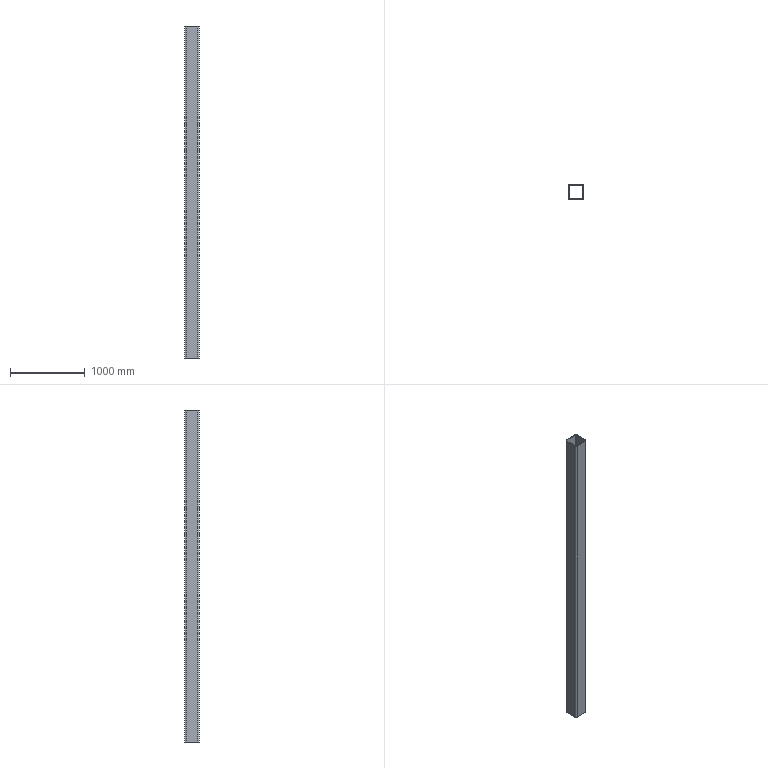Part | SolidWorks | features Extrusion 1 | 1 solid | 18 faces | box 200 x 200 x 4430 mm | volume 26244417 mm3 | plane 10 | cylinder 8 | commonest cylinder face diameters 24 x4 40 x4
STEP:
#1=CARTESIAN_POINT('',(-100.,-80.,4430.));
#2=VERTEX_POINT('',#1);
#3=CARTESIAN_POINT('',(-80.,-100.,4430.));
#4=VERTEX_POINT('',#3);
#5=CARTESIAN_POINT('',(-80.,-80.,4430.));
#6=DIRECTION('',(0.,0.,1.));
#7=DIRECTION('',(1.,0.,0.));
#8=AXIS2_PLACEMENT_3D('',#5,#6,#7);
#9=CIRCLE('',#8,20.);
#10=EDGE_CURVE('',#2,#4,#9,.T.);
#11=ORIENTED_EDGE('',*,*,#10,.T.);
#12=CARTESIAN_POINT('',(80.,-100.,4430.));
#13=VERTEX_POINT('',#12);
#14=CARTESIAN_POINT('',(-80.,-100.,4430.));
#15=DIRECTION('',(1.,0.,0.));
#16=VECTOR('',#15,1000.);
#17=LINE('',#14,#16);
#18=EDGE_CURVE('',#4,#13,#17,.T.);
#19=ORIENTED_EDGE('',*,*,#18,.T.);
#20=CARTESIAN_POINT('',(100.,-80.,4430.));
#21=VERTEX_POINT('',#20);
#22=CARTESIAN_POINT('',(80.,-80.,4430.));
#23=DIRECTION('',(0.,0.,1.));
#24=DIRECTION('',(1.,0.,0.));
#25=AXIS2_PLACEMENT_3D('',#22,#23,#24);
#26=CIRCLE('',#25,20.);
#27=EDGE_CURVE('',#13,#21,#26,.T.);
#28=ORIENTED_EDGE('',*,*,#27,.T.);
#29=CARTESIAN_POINT('',(100.,80.,4430.));
#30=VERTEX_POINT('',#29);
#31=CARTESIAN_POINT('',(100.,80.,4430.));
#32=DIRECTION('',(0.,1.,0.));
#33=VECTOR('',#32,1000.);
#34=LINE('',#31,#33);
#35=EDGE_CURVE('',#21,#30,#34,.T.);
#36=ORIENTED_EDGE('',*,*,#35,.T.);
#37=CARTESIAN_POINT('',(80.,100.,4430.));
#38=VERTEX_POINT('',#37);
#39=CARTESIAN_POINT('',(80.,80.,4430.));
#40=DIRECTION('',(0.,0.,1.));
#41=DIRECTION('',(-1.,0.,0.));
#42=AXIS2_PLACEMENT_3D('',#39,#40,#41);
#43=CIRCLE('',#42,20.);
#44=EDGE_CURVE('',#30,#38,#43,.T.);
#45=ORIENTED_EDGE('',*,*,#44,.T.);
#46=CARTESIAN_POINT('',(-80.,100.,4430.));
#47=VERTEX_POINT('',#46);
#48=CARTESIAN_POINT('',(-80.,100.,4430.));
#49=DIRECTION('',(-1.,0.,0.));
#50=VECTOR('',#49,1000.);
#51=LINE('',#48,#50);
#52=EDGE_CURVE('',#38,#47,#51,.T.);
#53=ORIENTED_EDGE('',*,*,#52,.T.);
#54=CARTESIAN_POINT('',(-100.,80.,4430.));
#55=VERTEX_POINT('',#54);
#56=CARTESIAN_POINT('',(-80.,80.,4430.));
#57=DIRECTION('',(0.,0.,1.));
#58=DIRECTION('',(1.,0.,0.));
#59=AXIS2_PLACEMENT_3D('',#56,#57,#58);
#60=CIRCLE('',#59,20.);
#61=EDGE_CURVE('',#47,#55,#60,.T.);
#62=ORIENTED_EDGE('',*,*,#61,.T.);
#63=CARTESIAN_POINT('',(-100.,80.,4430.));
#64=DIRECTION('',(0.,-1.,0.));
#65=VECTOR('',#64,1000.);
#66=LINE('',#63,#65);
#67=EDGE_CURVE('',#55,#2,#66,.T.);
#68=ORIENTED_EDGE('',*,*,#67,.T.);
#69=EDGE_LOOP('',(#11,#19,#28,#36,#45,#53,#62,#68));
#70=FACE_OUTER_BOUND('',#69,.T.);
#71=CARTESIAN_POINT('',(-92.,80.,4430.));
#72=VERTEX_POINT('',#71);
#73=CARTESIAN_POINT('',(-92.,-80.,4430.));
#74=VERTEX_POINT('',#73);
#75=CARTESIAN_POINT('',(-92.,80.,4430.));
#76=DIRECTION('',(0.,-1.,0.));
#77=VECTOR('',#76,1000.);
#78=LINE('',#75,#77);
#79=EDGE_CURVE('',#72,#74,#78,.T.);
#80=ORIENTED_EDGE('',*,*,#79,.F.);
#81=CARTESIAN_POINT('',(-80.,92.,4430.));
#82=VERTEX_POINT('',#81);
#83=CARTESIAN_POINT('',(-80.,80.,4430.));
#84=DIRECTION('',(0.,0.,1.));
#85=DIRECTION('',(1.,0.,0.));
#86=AXIS2_PLACEMENT_3D('',#83,#84,#85);
#87=CIRCLE('',#86,12.);
#88=EDGE_CURVE('',#82,#72,#87,.T.);
#89=ORIENTED_EDGE('',*,*,#88,.F.);
#90=CARTESIAN_POINT('',(80.,92.,4430.));
#91=VERTEX_POINT('',#90);
#92=CARTESIAN_POINT('',(-80.,92.,4430.));
#93=DIRECTION('',(-1.,0.,0.));
#94=VECTOR('',#93,1000.);
#95=LINE('',#92,#94);
#96=EDGE_CURVE('',#91,#82,#95,.T.);
#97=ORIENTED_EDGE('',*,*,#96,.F.);
#98=CARTESIAN_POINT('',(92.,80.,4430.));
#99=VERTEX_POINT('',#98);
#100=CARTESIAN_POINT('',(80.,80.,4430.));
#101=DIRECTION('',(0.,0.,1.));
#102=DIRECTION('',(-1.,0.,0.));
#103=AXIS2_PLACEMENT_3D('',#100,#101,#102);
#104=CIRCLE('',#103,12.);
#105=EDGE_CURVE('',#99,#91,#104,.T.);
#106=ORIENTED_EDGE('',*,*,#105,.F.);
#107=CARTESIAN_POINT('',(92.,-80.,4430.));
#108=VERTEX_POINT('',#107);
#109=CARTESIAN_POINT('',(92.,80.,4430.));
#110=DIRECTION('',(0.,1.,0.));
#111=VECTOR('',#110,1000.);
#112=LINE('',#109,#111);
#113=EDGE_CURVE('',#108,#99,#112,.T.);
#114=ORIENTED_EDGE('',*,*,#113,.F.);
#115=CARTESIAN_POINT('',(80.,-92.,4430.));
#116=VERTEX_POINT('',#115);
#117=CARTESIAN_POINT('',(80.,-80.,4430.));
#118=DIRECTION('',(0.,0.,1.));
#119=DIRECTION('',(1.,0.,0.));
#120=AXIS2_PLACEMENT_3D('',#117,#118,#119);
#121=CIRCLE('',#120,12.);
#122=EDGE_CURVE('',#116,#108,#121,.T.);
#123=ORIENTED_EDGE('',*,*,#122,.F.);
#124=CARTESIAN_POINT('',(-80.,-92.,4430.));
#125=VERTEX_POINT('',#124);
#126=CARTESIAN_POINT('',(-80.,-92.,4430.));
#127=DIRECTION('',(1.,0.,0.));
#128=VECTOR('',#127,1000.);
#129=LINE('',#126,#128);
#130=EDGE_CURVE('',#125,#116,#129,.T.);
#131=ORIENTED_EDGE('',*,*,#130,.F.);
#132=CARTESIAN_POINT('',(-80.,-80.,4430.));
#133=DIRECTION('',(0.,0.,1.));
#134=DIRECTION('',(1.,0.,0.));
#135=AXIS2_PLACEMENT_3D('',#132,#133,#134);
#136=CIRCLE('',#135,12.);
#137=EDGE_CURVE('',#74,#125,#136,.T.);
#138=ORIENTED_EDGE('',*,*,#137,.F.);
#139=EDGE_LOOP('',(#80,#89,#97,#106,#114,#123,#131,#138));
#140=FACE_BOUND('',#139,.T.);
#141=CARTESIAN_POINT('',(-80.,-80.,4430.));
#142=DIRECTION('',(0.,0.,1.));
#143=DIRECTION('',(1.,0.,0.));
#144=AXIS2_PLACEMENT_3D('',#141,#142,#143);
#145=PLANE('',#144);
#146=ADVANCED_FACE('',(#70,#140),#145,.T.);
#147=CARTESIAN_POINT('',(-100.,-80.,0.));
#148=VERTEX_POINT('',#147);
#149=CARTESIAN_POINT('',(-80.,-100.,0.));
#150=VERTEX_POINT('',#149);
#151=CARTESIAN_POINT('',(-80.,-80.,0.));
#152=DIRECTION('',(0.,0.,1.));
#153=DIRECTION('',(1.,0.,0.));
#154=AXIS2_PLACEMENT_3D('',#151,#152,#153);
#155=CIRCLE('',#154,20.);
#156=EDGE_CURVE('',#148,#150,#155,.T.);
#157=ORIENTED_EDGE('',*,*,#156,.F.);
#158=CARTESIAN_POINT('',(-100.,80.,0.));
#159=VERTEX_POINT('',#158);
#160=CARTESIAN_POINT('',(-100.,80.,0.));
#161=DIRECTION('',(0.,-1.,0.));
#162=VECTOR('',#161,1000.);
#163=LINE('',#160,#162);
#164=EDGE_CURVE('',#159,#148,#163,.T.);
#165=ORIENTED_EDGE('',*,*,#164,.F.);
#166=CARTESIAN_POINT('',(-80.,100.,0.));
#167=VERTEX_POINT('',#166);
#168=CARTESIAN_POINT('',(-80.,80.,0.));
#169=DIRECTION('',(0.,0.,1.));
#170=DIRECTION('',(1.,0.,0.));
#171=AXIS2_PLACEMENT_3D('',#168,#169,#170);
#172=CIRCLE('',#171,20.);
#173=EDGE_CURVE('',#167,#159,#172,.T.);
#174=ORIENTED_EDGE('',*,*,#173,.F.);
#175=CARTESIAN_POINT('',(80.,100.,0.));
#176=VERTEX_POINT('',#175);
#177=CARTESIAN_POINT('',(-80.,100.,0.));
#178=DIRECTION('',(-1.,0.,0.));
#179=VECTOR('',#178,1000.);
#180=LINE('',#177,#179);
#181=EDGE_CURVE('',#176,#167,#180,.T.);
#182=ORIENTED_EDGE('',*,*,#181,.F.);
#183=CARTESIAN_POINT('',(100.,80.,0.));
#184=VERTEX_POINT('',#183);
#185=CARTESIAN_POINT('',(80.,80.,0.));
#186=DIRECTION('',(0.,0.,1.));
#187=DIRECTION('',(-1.,0.,0.));
#188=AXIS2_PLACEMENT_3D('',#185,#186,#187);
#189=CIRCLE('',#188,20.);
#190=EDGE_CURVE('',#184,#176,#189,.T.);
#191=ORIENTED_EDGE('',*,*,#190,.F.);
#192=CARTESIAN_POINT('',(100.,-80.,0.));
#193=VERTEX_POINT('',#192);
#194=CARTESIAN_POINT('',(100.,80.,0.));
#195=DIRECTION('',(0.,1.,0.));
#196=VECTOR('',#195,1000.);
#197=LINE('',#194,#196);
#198=EDGE_CURVE('',#193,#184,#197,.T.);
#199=ORIENTED_EDGE('',*,*,#198,.F.);
#200=CARTESIAN_POINT('',(80.,-100.,0.));
#201=VERTEX_POINT('',#200);
#202=CARTESIAN_POINT('',(80.,-80.,0.));
#203=DIRECTION('',(0.,0.,1.));
#204=DIRECTION('',(1.,0.,0.));
#205=AXIS2_PLACEMENT_3D('',#202,#203,#204);
#206=CIRCLE('',#205,20.);
#207=EDGE_CURVE('',#201,#193,#206,.T.);
#208=ORIENTED_EDGE('',*,*,#207,.F.);
#209=CARTESIAN_POINT('',(-80.,-100.,0.));
#210=DIRECTION('',(1.,0.,0.));
#211=VECTOR('',#210,1000.);
#212=LINE('',#209,#211);
#213=EDGE_CURVE('',#150,#201,#212,.T.);
#214=ORIENTED_EDGE('',*,*,#213,.F.);
#215=EDGE_LOOP('',(#157,#165,#174,#182,#191,#199,#208,#214));
#216=FACE_OUTER_BOUND('',#215,.T.);
#217=CARTESIAN_POINT('',(-80.,92.,0.));
#218=VERTEX_POINT('',#217);
#219=CARTESIAN_POINT('',(-92.,80.,0.));
#220=VERTEX_POINT('',#219);
#221=CARTESIAN_POINT('',(-80.,80.,0.));
#222=DIRECTION('',(0.,0.,1.));
#223=DIRECTION('',(1.,0.,0.));
#224=AXIS2_PLACEMENT_3D('',#221,#222,#223);
#225=CIRCLE('',#224,12.);
#226=EDGE_CURVE('',#218,#220,#225,.T.);
#227=ORIENTED_EDGE('',*,*,#226,.T.);
#228=CARTESIAN_POINT('',(-92.,-80.,0.));
#229=VERTEX_POINT('',#228);
#230=CARTESIAN_POINT('',(-92.,80.,0.));
#231=DIRECTION('',(0.,-1.,0.));
#232=VECTOR('',#231,1000.);
#233=LINE('',#230,#232);
#234=EDGE_CURVE('',#220,#229,#233,.T.);
#235=ORIENTED_EDGE('',*,*,#234,.T.);
#236=CARTESIAN_POINT('',(-80.,-92.,0.));
#237=VERTEX_POINT('',#236);
#238=CARTESIAN_POINT('',(-80.,-80.,0.));
#239=DIRECTION('',(0.,0.,1.));
#240=DIRECTION('',(1.,0.,0.));
#241=AXIS2_PLACEMENT_3D('',#238,#239,#240);
#242=CIRCLE('',#241,12.);
#243=EDGE_CURVE('',#229,#237,#242,.T.);
#244=ORIENTED_EDGE('',*,*,#243,.T.);
#245=CARTESIAN_POINT('',(80.,-92.,0.));
#246=VERTEX_POINT('',#245);
#247=CARTESIAN_POINT('',(-80.,-92.,0.));
#248=DIRECTION('',(1.,0.,0.));
#249=VECTOR('',#248,1000.);
#250=LINE('',#247,#249);
#251=EDGE_CURVE('',#237,#246,#250,.T.);
#252=ORIENTED_EDGE('',*,*,#251,.T.);
#253=CARTESIAN_POINT('',(92.,-80.,0.));
#254=VERTEX_POINT('',#253);
#255=CARTESIAN_POINT('',(80.,-80.,0.));
#256=DIRECTION('',(0.,0.,1.));
#257=DIRECTION('',(1.,0.,0.));
#258=AXIS2_PLACEMENT_3D('',#255,#256,#257);
#259=CIRCLE('',#258,12.);
#260=EDGE_CURVE('',#246,#254,#259,.T.);
#261=ORIENTED_EDGE('',*,*,#260,.T.);
#262=CARTESIAN_POINT('',(92.,80.,0.));
#263=VERTEX_POINT('',#262);
#264=CARTESIAN_POINT('',(92.,80.,0.));
#265=DIRECTION('',(0.,1.,0.));
#266=VECTOR('',#265,1000.);
#267=LINE('',#264,#266);
#268=EDGE_CURVE('',#254,#263,#267,.T.);
#269=ORIENTED_EDGE('',*,*,#268,.T.);
#270=CARTESIAN_POINT('',(80.,92.,0.));
#271=VERTEX_POINT('',#270);
#272=CARTESIAN_POINT('',(80.,80.,0.));
#273=DIRECTION('',(0.,0.,1.));
#274=DIRECTION('',(-1.,0.,0.));
#275=AXIS2_PLACEMENT_3D('',#272,#273,#274);
#276=CIRCLE('',#275,12.);
#277=EDGE_CURVE('',#263,#271,#276,.T.);
#278=ORIENTED_EDGE('',*,*,#277,.T.);
#279=CARTESIAN_POINT('',(-80.,92.,0.));
#280=DIRECTION('',(-1.,0.,0.));
#281=VECTOR('',#280,1000.);
#282=LINE('',#279,#281);
#283=EDGE_CURVE('',#271,#218,#282,.T.);
#284=ORIENTED_EDGE('',*,*,#283,.T.);
#285=EDGE_LOOP('',(#227,#235,#244,#252,#261,#269,#278,#284));
#286=FACE_BOUND('',#285,.T.);
#287=CARTESIAN_POINT('',(-80.,-80.,0.));
#288=DIRECTION('',(0.,0.,1.));
#289=DIRECTION('',(1.,0.,0.));
#290=AXIS2_PLACEMENT_3D('',#287,#288,#289);
#291=PLANE('',#290);
#292=ADVANCED_FACE('',(#216,#286),#291,.F.);
#293=ORIENTED_EDGE('',*,*,#156,.T.);
#294=CARTESIAN_POINT('',(-80.,-100.,4430.));
#295=DIRECTION('',(0.,0.,-1.));
#296=VECTOR('',#295,1000.);
#297=LINE('',#294,#296);
#298=EDGE_CURVE('',#4,#150,#297,.T.);
#299=ORIENTED_EDGE('',*,*,#298,.F.);
#300=ORIENTED_EDGE('',*,*,#10,.F.);
#301=CARTESIAN_POINT('',(-100.,-80.,4430.));
#302=DIRECTION('',(0.,0.,-1.));
#303=VECTOR('',#302,1000.);
#304=LINE('',#301,#303);
#305=EDGE_CURVE('',#2,#148,#304,.T.);
#306=ORIENTED_EDGE('',*,*,#305,.T.);
#307=EDGE_LOOP('',(#293,#299,#300,#306));
#308=FACE_OUTER_BOUND('',#307,.T.);
#309=CARTESIAN_POINT('',(-80.,-80.,4430.));
#310=DIRECTION('',(0.,0.,-1.));
#311=DIRECTION('',(-1.,0.,0.));
#312=AXIS2_PLACEMENT_3D('',#309,#310,#311);
#313=CYLINDRICAL_SURFACE('',#312,20.);
#314=ADVANCED_FACE('',(#308),#313,.T.);
#315=ORIENTED_EDGE('',*,*,#213,.T.);
#316=CARTESIAN_POINT('',(80.,-100.,4430.));
#317=DIRECTION('',(0.,0.,-1.));
#318=VECTOR('',#317,1000.);
#319=LINE('',#316,#318);
#320=EDGE_CURVE('',#13,#201,#319,.T.);
#321=ORIENTED_EDGE('',*,*,#320,.F.);
#322=ORIENTED_EDGE('',*,*,#18,.F.);
#323=ORIENTED_EDGE('',*,*,#298,.T.);
#324=EDGE_LOOP('',(#315,#321,#322,#323));
#325=FACE_OUTER_BOUND('',#324,.T.);
#326=CARTESIAN_POINT('',(-80.,-100.,4430.));
#327=DIRECTION('',(0.,1.,0.));
#328=DIRECTION('',(0.,0.,1.));
#329=AXIS2_PLACEMENT_3D('',#326,#327,#328);
#330=PLANE('',#329);
#331=ADVANCED_FACE('',(#325),#330,.F.);
#332=ORIENTED_EDGE('',*,*,#207,.T.);
#333=CARTESIAN_POINT('',(100.,-80.,4430.));
#334=DIRECTION('',(0.,0.,-1.));
#335=VECTOR('',#334,1000.);
#336=LINE('',#333,#335);
#337=EDGE_CURVE('',#21,#193,#336,.T.);
#338=ORIENTED_EDGE('',*,*,#337,.F.);
#339=ORIENTED_EDGE('',*,*,#27,.F.);
#340=ORIENTED_EDGE('',*,*,#320,.T.);
#341=EDGE_LOOP('',(#332,#338,#339,#340));
#342=FACE_OUTER_BOUND('',#341,.T.);
#343=CARTESIAN_POINT('',(80.,-80.,4430.));
#344=DIRECTION('',(0.,0.,-1.));
#345=DIRECTION('',(-1.,0.,0.));
#346=AXIS2_PLACEMENT_3D('',#343,#344,#345);
#347=CYLINDRICAL_SURFACE('',#346,20.);
#348=ADVANCED_FACE('',(#342),#347,.T.);
#349=ORIENTED_EDGE('',*,*,#198,.T.);
#350=CARTESIAN_POINT('',(100.,80.,4430.));
#351=DIRECTION('',(0.,0.,-1.));
#352=VECTOR('',#351,1000.);
#353=LINE('',#350,#352);
#354=EDGE_CURVE('',#30,#184,#353,.T.);
#355=ORIENTED_EDGE('',*,*,#354,.F.);
#356=ORIENTED_EDGE('',*,*,#35,.F.);
#357=ORIENTED_EDGE('',*,*,#337,.T.);
#358=EDGE_LOOP('',(#349,#355,#356,#357));
#359=FACE_OUTER_BOUND('',#358,.T.);
#360=CARTESIAN_POINT('',(100.,80.,4430.));
#361=DIRECTION('',(-1.,0.,0.));
#362=DIRECTION('',(0.,-1.,0.));
#363=AXIS2_PLACEMENT_3D('',#360,#361,#362);
#364=PLANE('',#363);
#365=ADVANCED_FACE('',(#359),#364,.F.);
#366=ORIENTED_EDGE('',*,*,#190,.T.);
#367=CARTESIAN_POINT('',(80.,100.,4430.));
#368=DIRECTION('',(0.,0.,-1.));
#369=VECTOR('',#368,1000.);
#370=LINE('',#367,#369);
#371=EDGE_CURVE('',#38,#176,#370,.T.);
#372=ORIENTED_EDGE('',*,*,#371,.F.);
#373=ORIENTED_EDGE('',*,*,#44,.F.);
#374=ORIENTED_EDGE('',*,*,#354,.T.);
#375=EDGE_LOOP('',(#366,#372,#373,#374));
#376=FACE_OUTER_BOUND('',#375,.T.);
#377=CARTESIAN_POINT('',(80.,80.,4430.));
#378=DIRECTION('',(0.,0.,-1.));
#379=DIRECTION('',(-1.,0.,0.));
#380=AXIS2_PLACEMENT_3D('',#377,#378,#379);
#381=CYLINDRICAL_SURFACE('',#380,20.);
#382=ADVANCED_FACE('',(#376),#381,.T.);
#383=ORIENTED_EDGE('',*,*,#181,.T.);
#384=CARTESIAN_POINT('',(-80.,100.,4430.));
#385=DIRECTION('',(0.,0.,-1.));
#386=VECTOR('',#385,1000.);
#387=LINE('',#384,#386);
#388=EDGE_CURVE('',#47,#167,#387,.T.);
#389=ORIENTED_EDGE('',*,*,#388,.F.);
#390=ORIENTED_EDGE('',*,*,#52,.F.);
#391=ORIENTED_EDGE('',*,*,#371,.T.);
#392=EDGE_LOOP('',(#383,#389,#390,#391));
#393=FACE_OUTER_BOUND('',#392,.T.);
#394=CARTESIAN_POINT('',(-80.,100.,4430.));
#395=DIRECTION('',(0.,-1.,0.));
#396=DIRECTION('',(0.,0.,-1.));
#397=AXIS2_PLACEMENT_3D('',#394,#395,#396);
#398=PLANE('',#397);
#399=ADVANCED_FACE('',(#393),#398,.F.);
#400=ORIENTED_EDGE('',*,*,#173,.T.);
#401=CARTESIAN_POINT('',(-100.,80.,4430.));
#402=DIRECTION('',(0.,0.,-1.));
#403=VECTOR('',#402,1000.);
#404=LINE('',#401,#403);
#405=EDGE_CURVE('',#55,#159,#404,.T.);
#406=ORIENTED_EDGE('',*,*,#405,.F.);
#407=ORIENTED_EDGE('',*,*,#61,.F.);
#408=ORIENTED_EDGE('',*,*,#388,.T.);
#409=EDGE_LOOP('',(#400,#406,#407,#408));
#410=FACE_OUTER_BOUND('',#409,.T.);
#411=CARTESIAN_POINT('',(-80.,80.,4430.));
#412=DIRECTION('',(0.,0.,-1.));
#413=DIRECTION('',(-1.,0.,0.));
#414=AXIS2_PLACEMENT_3D('',#411,#412,#413);
#415=CYLINDRICAL_SURFACE('',#414,20.);
#416=ADVANCED_FACE('',(#410),#415,.T.);
#417=ORIENTED_EDGE('',*,*,#164,.T.);
#418=ORIENTED_EDGE('',*,*,#305,.F.);
#419=ORIENTED_EDGE('',*,*,#67,.F.);
#420=ORIENTED_EDGE('',*,*,#405,.T.);
#421=EDGE_LOOP('',(#417,#418,#419,#420));
#422=FACE_OUTER_BOUND('',#421,.T.);
#423=CARTESIAN_POINT('',(-100.,80.,4430.));
#424=DIRECTION('',(1.,0.,0.));
#425=DIRECTION('',(0.,1.,0.));
#426=AXIS2_PLACEMENT_3D('',#423,#424,#425);
#427=PLANE('',#426);
#428=ADVANCED_FACE('',(#422),#427,.F.);
#429=ORIENTED_EDGE('',*,*,#226,.F.);
#430=CARTESIAN_POINT('',(-80.,92.,4430.));
#431=DIRECTION('',(0.,0.,-1.));
#432=VECTOR('',#431,1000.);
#433=LINE('',#430,#432);
#434=EDGE_CURVE('',#82,#218,#433,.T.);
#435=ORIENTED_EDGE('',*,*,#434,.F.);
#436=ORIENTED_EDGE('',*,*,#88,.T.);
#437=CARTESIAN_POINT('',(-92.,80.,4430.));
#438=DIRECTION('',(0.,0.,-1.));
#439=VECTOR('',#438,1000.);
#440=LINE('',#437,#439);
#441=EDGE_CURVE('',#72,#220,#440,.T.);
#442=ORIENTED_EDGE('',*,*,#441,.T.);
#443=EDGE_LOOP('',(#429,#435,#436,#442));
#444=FACE_OUTER_BOUND('',#443,.T.);
#445=CARTESIAN_POINT('',(-80.,80.,4430.));
#446=DIRECTION('',(0.,0.,-1.));
#447=DIRECTION('',(-1.,0.,0.));
#448=AXIS2_PLACEMENT_3D('',#445,#446,#447);
#449=CYLINDRICAL_SURFACE('',#448,12.);
#450=ADVANCED_FACE('',(#444),#449,.F.);
#451=ORIENTED_EDGE('',*,*,#234,.F.);
#452=ORIENTED_EDGE('',*,*,#441,.F.);
#453=ORIENTED_EDGE('',*,*,#79,.T.);
#454=CARTESIAN_POINT('',(-92.,-80.,4430.));
#455=DIRECTION('',(0.,0.,-1.));
#456=VECTOR('',#455,1000.);
#457=LINE('',#454,#456);
#458=EDGE_CURVE('',#74,#229,#457,.T.);
#459=ORIENTED_EDGE('',*,*,#458,.T.);
#460=EDGE_LOOP('',(#451,#452,#453,#459));
#461=FACE_OUTER_BOUND('',#460,.T.);
#462=CARTESIAN_POINT('',(-92.,80.,4430.));
#463=DIRECTION('',(1.,0.,0.));
#464=DIRECTION('',(0.,0.,-1.));
#465=AXIS2_PLACEMENT_3D('',#462,#463,#464);
#466=PLANE('',#465);
#467=ADVANCED_FACE('',(#461),#466,.T.);
#468=ORIENTED_EDGE('',*,*,#243,.F.);
#469=ORIENTED_EDGE('',*,*,#458,.F.);
#470=ORIENTED_EDGE('',*,*,#137,.T.);
#471=CARTESIAN_POINT('',(-80.,-92.,4430.));
#472=DIRECTION('',(0.,0.,-1.));
#473=VECTOR('',#472,1000.);
#474=LINE('',#471,#473);
#475=EDGE_CURVE('',#125,#237,#474,.T.);
#476=ORIENTED_EDGE('',*,*,#475,.T.);
#477=EDGE_LOOP('',(#468,#469,#470,#476));
#478=FACE_OUTER_BOUND('',#477,.T.);
#479=CARTESIAN_POINT('',(-80.,-80.,4430.));
#480=DIRECTION('',(0.,0.,-1.));
#481=DIRECTION('',(-1.,0.,0.));
#482=AXIS2_PLACEMENT_3D('',#479,#480,#481);
#483=CYLINDRICAL_SURFACE('',#482,12.);
#484=ADVANCED_FACE('',(#478),#483,.F.);
#485=ORIENTED_EDGE('',*,*,#251,.F.);
#486=ORIENTED_EDGE('',*,*,#475,.F.);
#487=ORIENTED_EDGE('',*,*,#130,.T.);
#488=CARTESIAN_POINT('',(80.,-92.,4430.));
#489=DIRECTION('',(0.,0.,-1.));
#490=VECTOR('',#489,1000.);
#491=LINE('',#488,#490);
#492=EDGE_CURVE('',#116,#246,#491,.T.);
#493=ORIENTED_EDGE('',*,*,#492,.T.);
#494=EDGE_LOOP('',(#485,#486,#487,#493));
#495=FACE_OUTER_BOUND('',#494,.T.);
#496=CARTESIAN_POINT('',(-80.,-92.,4430.));
#497=DIRECTION('',(0.,1.,0.));
#498=DIRECTION('',(0.,0.,1.));
#499=AXIS2_PLACEMENT_3D('',#496,#497,#498);
#500=PLANE('',#499);
#501=ADVANCED_FACE('',(#495),#500,.T.);
#502=ORIENTED_EDGE('',*,*,#260,.F.);
#503=ORIENTED_EDGE('',*,*,#492,.F.);
#504=ORIENTED_EDGE('',*,*,#122,.T.);
#505=CARTESIAN_POINT('',(92.,-80.,4430.));
#506=DIRECTION('',(0.,0.,-1.));
#507=VECTOR('',#506,1000.);
#508=LINE('',#505,#507);
#509=EDGE_CURVE('',#108,#254,#508,.T.);
#510=ORIENTED_EDGE('',*,*,#509,.T.);
#511=EDGE_LOOP('',(#502,#503,#504,#510));
#512=FACE_OUTER_BOUND('',#511,.T.);
#513=CARTESIAN_POINT('',(80.,-80.,4430.));
#514=DIRECTION('',(0.,0.,-1.));
#515=DIRECTION('',(-1.,0.,0.));
#516=AXIS2_PLACEMENT_3D('',#513,#514,#515);
#517=CYLINDRICAL_SURFACE('',#516,12.);
#518=ADVANCED_FACE('',(#512),#517,.F.);
#519=ORIENTED_EDGE('',*,*,#268,.F.);
#520=ORIENTED_EDGE('',*,*,#509,.F.);
#521=ORIENTED_EDGE('',*,*,#113,.T.);
#522=CARTESIAN_POINT('',(92.,80.,4430.));
#523=DIRECTION('',(0.,0.,-1.));
#524=VECTOR('',#523,1000.);
#525=LINE('',#522,#524);
#526=EDGE_CURVE('',#99,#263,#525,.T.);
#527=ORIENTED_EDGE('',*,*,#526,.T.);
#528=EDGE_LOOP('',(#519,#520,#521,#527));
#529=FACE_OUTER_BOUND('',#528,.T.);
#530=CARTESIAN_POINT('',(92.,80.,4430.));
#531=DIRECTION('',(-1.,0.,0.));
#532=DIRECTION('',(0.,-1.,0.));
#533=AXIS2_PLACEMENT_3D('',#530,#531,#532);
#534=PLANE('',#533);
#535=ADVANCED_FACE('',(#529),#534,.T.);
#536=ORIENTED_EDGE('',*,*,#277,.F.);
#537=ORIENTED_EDGE('',*,*,#526,.F.);
#538=ORIENTED_EDGE('',*,*,#105,.T.);
#539=CARTESIAN_POINT('',(80.,92.,4430.));
#540=DIRECTION('',(0.,0.,-1.));
#541=VECTOR('',#540,1000.);
#542=LINE('',#539,#541);
#543=EDGE_CURVE('',#91,#271,#542,.T.);
#544=ORIENTED_EDGE('',*,*,#543,.T.);
#545=EDGE_LOOP('',(#536,#537,#538,#544));
#546=FACE_OUTER_BOUND('',#545,.T.);
#547=CARTESIAN_POINT('',(80.,80.,4430.));
#548=DIRECTION('',(0.,0.,-1.));
#549=DIRECTION('',(-1.,0.,0.));
#550=AXIS2_PLACEMENT_3D('',#547,#548,#549);
#551=CYLINDRICAL_SURFACE('',#550,12.);
#552=ADVANCED_FACE('',(#546),#551,.F.);
#553=ORIENTED_EDGE('',*,*,#283,.F.);
#554=ORIENTED_EDGE('',*,*,#543,.F.);
#555=ORIENTED_EDGE('',*,*,#96,.T.);
#556=ORIENTED_EDGE('',*,*,#434,.T.);
#557=EDGE_LOOP('',(#553,#554,#555,#556));
#558=FACE_OUTER_BOUND('',#557,.T.);
#559=CARTESIAN_POINT('',(-80.,92.,4430.));
#560=DIRECTION('',(0.,-1.,0.));
#561=DIRECTION('',(0.,0.,-1.));
#562=AXIS2_PLACEMENT_3D('',#559,#560,#561);
#563=PLANE('',#562);
#564=ADVANCED_FACE('',(#558),#563,.T.);
#565=CLOSED_SHELL('',(#146,#292,#314,#331,#348,#365,#382,#399,#416,#428,#450,#467,#484,#501,#518,#535,#552,#564));
#566=MANIFOLD_SOLID_BREP('',#565);
#567=CARTESIAN_POINT('',(0.,0.,0.));
#568=DIRECTION('',(0.,0.,1.));
#569=DIRECTION('',(1.,0.,0.));
#570=AXIS2_PLACEMENT_3D('',#567,#568,#569);
#571=(LENGTH_UNIT()NAMED_UNIT(*)SI_UNIT(.MILLI.,.METRE.));
#572=UNCERTAINTY_MEASURE_WITH_UNIT(LENGTH_MEASURE(0.00001),#571,'','');
#573=(NAMED_UNIT(*)PLANE_ANGLE_UNIT()SI_UNIT($,.RADIAN.));
#574=(NAMED_UNIT(*)SI_UNIT($,.STERADIAN.)SOLID_ANGLE_UNIT());
#575=(GEOMETRIC_REPRESENTATION_CONTEXT(3)GLOBAL_UNCERTAINTY_ASSIGNED_CONTEXT((#572))GLOBAL_UNIT_ASSIGNED_CONTEXT((#571,#573,#574))REPRESENTATION_CONTEXT('',''));
#576=ADVANCED_BREP_SHAPE_REPRESENTATION('',(#566,#570),#575);